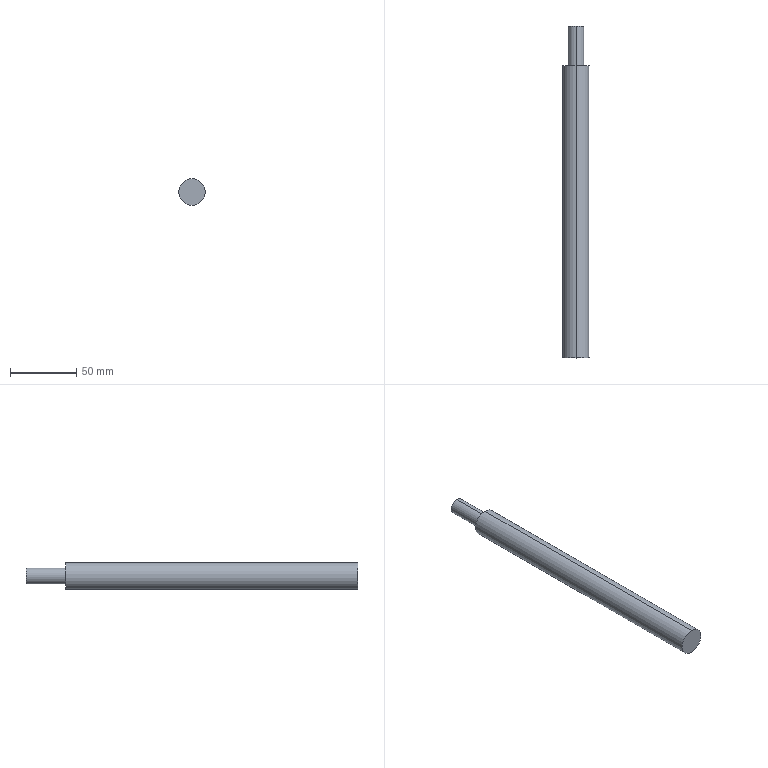Part | SolidWorks | features Cut 1, Extrusion 1 | 1 solid | 7 faces | box 20 x 250 x 20 mm | volume 72508 mm3 | cylinder 4 | plane 3 | commonest cylinder face diameters 12 x2 20 x2
STEP:
#1=CARTESIAN_POINT('',(0.,220.,6.));
#2=VERTEX_POINT('',#1);
#3=CARTESIAN_POINT('',(0.,220.,-6.));
#4=VERTEX_POINT('',#3);
#5=CARTESIAN_POINT('',(0.,220.,0.));
#6=DIRECTION('',(0.,1.,0.));
#7=DIRECTION('',(0.,0.,1.));
#8=AXIS2_PLACEMENT_3D('',#5,#6,#7);
#9=CIRCLE('',#8,6.);
#10=EDGE_CURVE('',#2,#4,#9,.T.);
#11=ORIENTED_EDGE('',*,*,#10,.T.);
#12=CARTESIAN_POINT('',(0.,250.,-6.));
#13=VERTEX_POINT('',#12);
#14=CARTESIAN_POINT('',(0.,220.,-6.));
#15=DIRECTION('',(0.,1.,0.));
#16=VECTOR('',#15,1000.);
#17=LINE('',#14,#16);
#18=EDGE_CURVE('',#4,#13,#17,.T.);
#19=ORIENTED_EDGE('',*,*,#18,.T.);
#20=CARTESIAN_POINT('',(0.,250.,6.));
#21=VERTEX_POINT('',#20);
#22=CARTESIAN_POINT('',(0.,250.,0.));
#23=DIRECTION('',(0.,1.,0.));
#24=DIRECTION('',(0.,0.,1.));
#25=AXIS2_PLACEMENT_3D('',#22,#23,#24);
#26=CIRCLE('',#25,6.);
#27=EDGE_CURVE('',#21,#13,#26,.T.);
#28=ORIENTED_EDGE('',*,*,#27,.F.);
#29=CARTESIAN_POINT('',(0.,220.,6.));
#30=DIRECTION('',(0.,1.,0.));
#31=VECTOR('',#30,1000.);
#32=LINE('',#29,#31);
#33=EDGE_CURVE('',#2,#21,#32,.T.);
#34=ORIENTED_EDGE('',*,*,#33,.F.);
#35=EDGE_LOOP('',(#11,#19,#28,#34));
#36=FACE_OUTER_BOUND('',#35,.T.);
#37=CARTESIAN_POINT('',(0.,220.,0.));
#38=DIRECTION('',(0.,1.,0.));
#39=DIRECTION('',(0.,0.,1.));
#40=AXIS2_PLACEMENT_3D('',#37,#38,#39);
#41=CYLINDRICAL_SURFACE('',#40,6.);
#42=ADVANCED_FACE('',(#36),#41,.T.);
#43=CARTESIAN_POINT('',(0.,220.,10.));
#44=VERTEX_POINT('',#43);
#45=CARTESIAN_POINT('',(0.,220.,-10.));
#46=VERTEX_POINT('',#45);
#47=CARTESIAN_POINT('',(0.,220.,0.));
#48=DIRECTION('',(0.,1.,0.));
#49=DIRECTION('',(0.,0.,1.));
#50=AXIS2_PLACEMENT_3D('',#47,#48,#49);
#51=CIRCLE('',#50,10.);
#52=EDGE_CURVE('',#44,#46,#51,.T.);
#53=ORIENTED_EDGE('',*,*,#52,.F.);
#54=CARTESIAN_POINT('',(0.,0.,10.));
#55=VERTEX_POINT('',#54);
#56=CARTESIAN_POINT('',(0.,250.,10.));
#57=DIRECTION('',(0.,-1.,0.));
#58=VECTOR('',#57,1000.);
#59=LINE('',#56,#58);
#60=EDGE_CURVE('',#44,#55,#59,.T.);
#61=ORIENTED_EDGE('',*,*,#60,.T.);
#62=CARTESIAN_POINT('',(0.,0.,-10.));
#63=VERTEX_POINT('',#62);
#64=CARTESIAN_POINT('',(0.,0.,0.));
#65=DIRECTION('',(0.,1.,0.));
#66=DIRECTION('',(0.,0.,1.));
#67=AXIS2_PLACEMENT_3D('',#64,#65,#66);
#68=CIRCLE('',#67,10.);
#69=EDGE_CURVE('',#55,#63,#68,.T.);
#70=ORIENTED_EDGE('',*,*,#69,.T.);
#71=CARTESIAN_POINT('',(0.,250.,-10.));
#72=DIRECTION('',(0.,-1.,0.));
#73=VECTOR('',#72,1000.);
#74=LINE('',#71,#73);
#75=EDGE_CURVE('',#46,#63,#74,.T.);
#76=ORIENTED_EDGE('',*,*,#75,.F.);
#77=EDGE_LOOP('',(#53,#61,#70,#76));
#78=FACE_OUTER_BOUND('',#77,.T.);
#79=CARTESIAN_POINT('',(0.,250.,0.));
#80=DIRECTION('',(0.,-1.,0.));
#81=DIRECTION('',(0.,0.,-1.));
#82=AXIS2_PLACEMENT_3D('',#79,#80,#81);
#83=CYLINDRICAL_SURFACE('',#82,10.);
#84=ADVANCED_FACE('',(#78),#83,.T.);
#85=ORIENTED_EDGE('',*,*,#60,.F.);
#86=CARTESIAN_POINT('',(0.,220.,0.));
#87=DIRECTION('',(0.,1.,0.));
#88=DIRECTION('',(0.,0.,1.));
#89=AXIS2_PLACEMENT_3D('',#86,#87,#88);
#90=CIRCLE('',#89,10.);
#91=EDGE_CURVE('',#46,#44,#90,.T.);
#92=ORIENTED_EDGE('',*,*,#91,.F.);
#93=ORIENTED_EDGE('',*,*,#75,.T.);
#94=CARTESIAN_POINT('',(0.,0.,0.));
#95=DIRECTION('',(0.,1.,0.));
#96=DIRECTION('',(0.,0.,1.));
#97=AXIS2_PLACEMENT_3D('',#94,#95,#96);
#98=CIRCLE('',#97,10.);
#99=EDGE_CURVE('',#63,#55,#98,.T.);
#100=ORIENTED_EDGE('',*,*,#99,.T.);
#101=EDGE_LOOP('',(#85,#92,#93,#100));
#102=FACE_OUTER_BOUND('',#101,.T.);
#103=CARTESIAN_POINT('',(0.,250.,0.));
#104=DIRECTION('',(0.,-1.,0.));
#105=DIRECTION('',(0.,0.,-1.));
#106=AXIS2_PLACEMENT_3D('',#103,#104,#105);
#107=CYLINDRICAL_SURFACE('',#106,10.);
#108=ADVANCED_FACE('',(#102),#107,.T.);
#109=ORIENTED_EDGE('',*,*,#99,.F.);
#110=ORIENTED_EDGE('',*,*,#69,.F.);
#111=EDGE_LOOP('',(#109,#110));
#112=FACE_OUTER_BOUND('',#111,.T.);
#113=CARTESIAN_POINT('',(0.,0.,0.));
#114=DIRECTION('',(0.,1.,0.));
#115=DIRECTION('',(0.,0.,1.));
#116=AXIS2_PLACEMENT_3D('',#113,#114,#115);
#117=PLANE('',#116);
#118=ADVANCED_FACE('',(#112),#117,.F.);
#119=ORIENTED_EDGE('',*,*,#10,.F.);
#120=CARTESIAN_POINT('',(0.,220.,0.));
#121=DIRECTION('',(0.,1.,0.));
#122=DIRECTION('',(0.,0.,1.));
#123=AXIS2_PLACEMENT_3D('',#120,#121,#122);
#124=CIRCLE('',#123,6.);
#125=EDGE_CURVE('',#4,#2,#124,.T.);
#126=ORIENTED_EDGE('',*,*,#125,.F.);
#127=EDGE_LOOP('',(#119,#126));
#128=FACE_BOUND('',#127,.T.);
#129=ORIENTED_EDGE('',*,*,#91,.T.);
#130=ORIENTED_EDGE('',*,*,#52,.T.);
#131=EDGE_LOOP('',(#129,#130));
#132=FACE_OUTER_BOUND('',#131,.T.);
#133=CARTESIAN_POINT('',(0.,220.,0.));
#134=DIRECTION('',(0.,1.,0.));
#135=DIRECTION('',(0.,0.,1.));
#136=AXIS2_PLACEMENT_3D('',#133,#134,#135);
#137=PLANE('',#136);
#138=ADVANCED_FACE('',(#128,#132),#137,.T.);
#139=ORIENTED_EDGE('',*,*,#18,.F.);
#140=ORIENTED_EDGE('',*,*,#125,.T.);
#141=ORIENTED_EDGE('',*,*,#33,.T.);
#142=CARTESIAN_POINT('',(0.,250.,0.));
#143=DIRECTION('',(0.,1.,0.));
#144=DIRECTION('',(0.,0.,1.));
#145=AXIS2_PLACEMENT_3D('',#142,#143,#144);
#146=CIRCLE('',#145,6.);
#147=EDGE_CURVE('',#13,#21,#146,.T.);
#148=ORIENTED_EDGE('',*,*,#147,.F.);
#149=EDGE_LOOP('',(#139,#140,#141,#148));
#150=FACE_OUTER_BOUND('',#149,.T.);
#151=CARTESIAN_POINT('',(0.,220.,0.));
#152=DIRECTION('',(0.,1.,0.));
#153=DIRECTION('',(0.,0.,1.));
#154=AXIS2_PLACEMENT_3D('',#151,#152,#153);
#155=CYLINDRICAL_SURFACE('',#154,6.);
#156=ADVANCED_FACE('',(#150),#155,.T.);
#157=ORIENTED_EDGE('',*,*,#27,.T.);
#158=ORIENTED_EDGE('',*,*,#147,.T.);
#159=EDGE_LOOP('',(#157,#158));
#160=FACE_OUTER_BOUND('',#159,.T.);
#161=CARTESIAN_POINT('',(0.,250.,0.));
#162=DIRECTION('',(0.,1.,0.));
#163=DIRECTION('',(0.,0.,1.));
#164=AXIS2_PLACEMENT_3D('',#161,#162,#163);
#165=PLANE('',#164);
#166=ADVANCED_FACE('',(#160),#165,.T.);
#167=CLOSED_SHELL('',(#42,#84,#108,#118,#138,#156,#166));
#168=MANIFOLD_SOLID_BREP('',#167);
#169=CARTESIAN_POINT('',(0.,0.,0.));
#170=DIRECTION('',(0.,0.,1.));
#171=DIRECTION('',(1.,0.,0.));
#172=AXIS2_PLACEMENT_3D('',#169,#170,#171);
#173=(LENGTH_UNIT()NAMED_UNIT(*)SI_UNIT(.MILLI.,.METRE.));
#174=UNCERTAINTY_MEASURE_WITH_UNIT(LENGTH_MEASURE(0.00001),#173,'','');
#175=(NAMED_UNIT(*)PLANE_ANGLE_UNIT()SI_UNIT($,.RADIAN.));
#176=(NAMED_UNIT(*)SI_UNIT($,.STERADIAN.)SOLID_ANGLE_UNIT());
#177=(GEOMETRIC_REPRESENTATION_CONTEXT(3)GLOBAL_UNCERTAINTY_ASSIGNED_CONTEXT((#174))GLOBAL_UNIT_ASSIGNED_CONTEXT((#173,#175,#176))REPRESENTATION_CONTEXT('',''));
#178=ADVANCED_BREP_SHAPE_REPRESENTATION('',(#168,#172),#177);